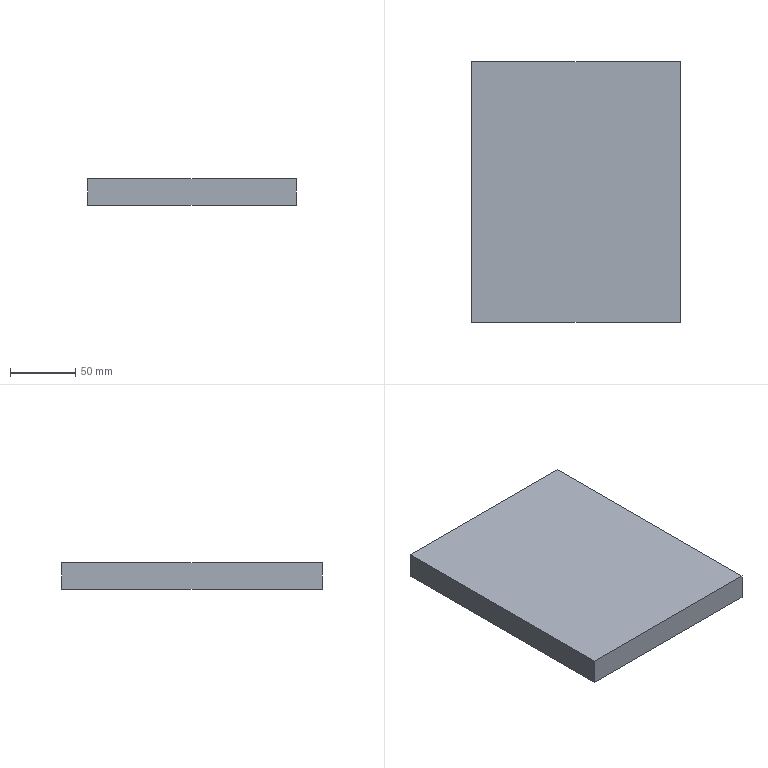Part | STEP file | Tube necking machine_id546_x_t | 1 solid | 6 faces | box 160 x 200 x 20 mm | volume 640000 mm3 | plane 6
STEP:
#1=CARTESIAN_POINT('',(0.,0.,0.));
#2=DIRECTION('',(0.,0.,1.));
#3=DIRECTION('',(1.,0.,0.));
#4=AXIS2_PLACEMENT_3D('',#1,#2,#3);
#5=CARTESIAN_POINT('',(387.5,150.,0.));
#6=VERTEX_POINT('',#5);
#7=CARTESIAN_POINT('',(387.5,-50.,0.));
#8=VERTEX_POINT('',#7);
#9=CARTESIAN_POINT('',(387.5,150.,0.));
#10=DIRECTION('',(0.,-1.,0.));
#11=VECTOR('',#10,1.);
#12=LINE('',#9,#11);
#13=CARTESIAN_POINT('',(387.5,150.,20.));
#14=DIRECTION('',(1.,0.,0.));
#15=DIRECTION('',(0.,0.,-1.));
#16=AXIS2_PLACEMENT_3D('',#13,#14,#15);
#17=PLANE('',#16);
#18=CARTESIAN_POINT('',(20.,0.));
#19=DIRECTION('',(0.,-1.));
#20=VECTOR('',#19,1.);
#21=LINE('',#18,#20);
#22=(GEOMETRIC_REPRESENTATION_CONTEXT(2)PARAMETRIC_REPRESENTATION_CONTEXT()REPRESENTATION_CONTEXT('',''));
#23=DEFINITIONAL_REPRESENTATION('',(#21),#22);
#24=PCURVE('',#17,#23);
#25=CARTESIAN_POINT('',(0.,0.,0.));
#26=DIRECTION('',(0.,0.,1.));
#27=DIRECTION('',(1.,0.,0.));
#28=AXIS2_PLACEMENT_3D('',#25,#26,#27);
#29=PLANE('',#28);
#30=CARTESIAN_POINT('',(387.5,150.));
#31=DIRECTION('',(0.,-1.));
#32=VECTOR('',#31,1.);
#33=LINE('',#30,#32);
#34=(GEOMETRIC_REPRESENTATION_CONTEXT(2)PARAMETRIC_REPRESENTATION_CONTEXT()REPRESENTATION_CONTEXT('',''));
#35=DEFINITIONAL_REPRESENTATION('',(#33),#34);
#36=PCURVE('',#29,#35);
#37=SURFACE_CURVE('',#12,(#24,#36),.PCURVE_S1.);
#38=EDGE_CURVE('',#6,#8,#37,.T.);
#39=ORIENTED_EDGE('',*,*,#38,.T.);
#40=CARTESIAN_POINT('',(387.5,-50.,20.));
#41=VERTEX_POINT('',#40);
#42=CARTESIAN_POINT('',(387.5,-50.,20.));
#43=DIRECTION('',(0.,0.,-1.));
#44=VECTOR('',#43,1.);
#45=LINE('',#42,#44);
#46=CARTESIAN_POINT('',(0.,-200.));
#47=DIRECTION('',(1.,0.));
#48=VECTOR('',#47,1.);
#49=LINE('',#46,#48);
#50=(GEOMETRIC_REPRESENTATION_CONTEXT(2)PARAMETRIC_REPRESENTATION_CONTEXT()REPRESENTATION_CONTEXT('',''));
#51=DEFINITIONAL_REPRESENTATION('',(#49),#50);
#52=PCURVE('',#17,#51);
#53=CARTESIAN_POINT('',(387.5,-50.,20.));
#54=DIRECTION('',(0.,1.,0.));
#55=DIRECTION('',(-1.,0.,0.));
#56=AXIS2_PLACEMENT_3D('',#53,#54,#55);
#57=PLANE('',#56);
#58=CARTESIAN_POINT('',(0.,0.));
#59=DIRECTION('',(0.,-1.));
#60=VECTOR('',#59,1.);
#61=LINE('',#58,#60);
#62=(GEOMETRIC_REPRESENTATION_CONTEXT(2)PARAMETRIC_REPRESENTATION_CONTEXT()REPRESENTATION_CONTEXT('',''));
#63=DEFINITIONAL_REPRESENTATION('',(#61),#62);
#64=PCURVE('',#57,#63);
#65=SURFACE_CURVE('',#45,(#52,#64),.PCURVE_S1.);
#66=EDGE_CURVE('',#41,#8,#65,.T.);
#67=ORIENTED_EDGE('',*,*,#66,.F.);
#68=CARTESIAN_POINT('',(387.5,150.,20.));
#69=VERTEX_POINT('',#68);
#70=CARTESIAN_POINT('',(387.5,150.,20.));
#71=DIRECTION('',(0.,-1.,0.));
#72=VECTOR('',#71,1.);
#73=LINE('',#70,#72);
#74=CARTESIAN_POINT('',(0.,0.));
#75=DIRECTION('',(0.,-1.));
#76=VECTOR('',#75,1.);
#77=LINE('',#74,#76);
#78=(GEOMETRIC_REPRESENTATION_CONTEXT(2)PARAMETRIC_REPRESENTATION_CONTEXT()REPRESENTATION_CONTEXT('',''));
#79=DEFINITIONAL_REPRESENTATION('',(#77),#78);
#80=PCURVE('',#17,#79);
#81=CARTESIAN_POINT('',(0.,0.,20.));
#82=DIRECTION('',(0.,0.,1.));
#83=DIRECTION('',(1.,0.,0.));
#84=AXIS2_PLACEMENT_3D('',#81,#82,#83);
#85=PLANE('',#84);
#86=CARTESIAN_POINT('',(387.5,150.));
#87=DIRECTION('',(0.,-1.));
#88=VECTOR('',#87,1.);
#89=LINE('',#86,#88);
#90=(GEOMETRIC_REPRESENTATION_CONTEXT(2)PARAMETRIC_REPRESENTATION_CONTEXT()REPRESENTATION_CONTEXT('',''));
#91=DEFINITIONAL_REPRESENTATION('',(#89),#90);
#92=PCURVE('',#85,#91);
#93=SURFACE_CURVE('',#73,(#80,#92),.PCURVE_S1.);
#94=EDGE_CURVE('',#69,#41,#93,.T.);
#95=ORIENTED_EDGE('',*,*,#94,.F.);
#96=CARTESIAN_POINT('',(387.5,150.,20.));
#97=DIRECTION('',(0.,0.,-1.));
#98=VECTOR('',#97,1.);
#99=LINE('',#96,#98);
#100=CARTESIAN_POINT('',(0.,0.));
#101=DIRECTION('',(1.,0.));
#102=VECTOR('',#101,1.);
#103=LINE('',#100,#102);
#104=(GEOMETRIC_REPRESENTATION_CONTEXT(2)PARAMETRIC_REPRESENTATION_CONTEXT()REPRESENTATION_CONTEXT('',''));
#105=DEFINITIONAL_REPRESENTATION('',(#103),#104);
#106=PCURVE('',#17,#105);
#107=CARTESIAN_POINT('',(547.5,150.,20.));
#108=DIRECTION('',(0.,-1.,0.));
#109=DIRECTION('',(0.,0.,-1.));
#110=AXIS2_PLACEMENT_3D('',#107,#108,#109);
#111=PLANE('',#110);
#112=CARTESIAN_POINT('',(0.,-160.));
#113=DIRECTION('',(1.,0.));
#114=VECTOR('',#113,1.);
#115=LINE('',#112,#114);
#116=(GEOMETRIC_REPRESENTATION_CONTEXT(2)PARAMETRIC_REPRESENTATION_CONTEXT()REPRESENTATION_CONTEXT('',''));
#117=DEFINITIONAL_REPRESENTATION('',(#115),#116);
#118=PCURVE('',#111,#117);
#119=SURFACE_CURVE('',#99,(#106,#118),.PCURVE_S1.);
#120=EDGE_CURVE('',#69,#6,#119,.T.);
#121=ORIENTED_EDGE('',*,*,#120,.T.);
#122=EDGE_LOOP('',(#39,#67,#95,#121));
#123=FACE_BOUND('',#122,.T.);
#124=ADVANCED_FACE('',(#123),#17,.F.);
#125=CARTESIAN_POINT('',(547.5,-50.,0.));
#126=VERTEX_POINT('',#125);
#127=CARTESIAN_POINT('',(387.5,-50.,0.));
#128=DIRECTION('',(1.,0.,0.));
#129=VECTOR('',#128,1.);
#130=LINE('',#127,#129);
#131=CARTESIAN_POINT('',(0.,-20.));
#132=DIRECTION('',(-1.,0.));
#133=VECTOR('',#132,1.);
#134=LINE('',#131,#133);
#135=(GEOMETRIC_REPRESENTATION_CONTEXT(2)PARAMETRIC_REPRESENTATION_CONTEXT()REPRESENTATION_CONTEXT('',''));
#136=DEFINITIONAL_REPRESENTATION('',(#134),#135);
#137=PCURVE('',#57,#136);
#138=CARTESIAN_POINT('',(387.5,-50.));
#139=DIRECTION('',(1.,0.));
#140=VECTOR('',#139,1.);
#141=LINE('',#138,#140);
#142=(GEOMETRIC_REPRESENTATION_CONTEXT(2)PARAMETRIC_REPRESENTATION_CONTEXT()REPRESENTATION_CONTEXT('',''));
#143=DEFINITIONAL_REPRESENTATION('',(#141),#142);
#144=PCURVE('',#29,#143);
#145=SURFACE_CURVE('',#130,(#137,#144),.PCURVE_S1.);
#146=EDGE_CURVE('',#8,#126,#145,.T.);
#147=ORIENTED_EDGE('',*,*,#146,.T.);
#148=CARTESIAN_POINT('',(547.5,-50.,20.));
#149=VERTEX_POINT('',#148);
#150=CARTESIAN_POINT('',(547.5,-50.,20.));
#151=DIRECTION('',(0.,0.,-1.));
#152=VECTOR('',#151,1.);
#153=LINE('',#150,#152);
#154=CARTESIAN_POINT('',(-160.,0.));
#155=DIRECTION('',(0.,-1.));
#156=VECTOR('',#155,1.);
#157=LINE('',#154,#156);
#158=(GEOMETRIC_REPRESENTATION_CONTEXT(2)PARAMETRIC_REPRESENTATION_CONTEXT()REPRESENTATION_CONTEXT('',''));
#159=DEFINITIONAL_REPRESENTATION('',(#157),#158);
#160=PCURVE('',#57,#159);
#161=CARTESIAN_POINT('',(547.5,-50.,20.));
#162=DIRECTION('',(-1.,0.,0.));
#163=DIRECTION('',(0.,-1.,0.));
#164=AXIS2_PLACEMENT_3D('',#161,#162,#163);
#165=PLANE('',#164);
#166=CARTESIAN_POINT('',(0.,0.));
#167=DIRECTION('',(0.,-1.));
#168=VECTOR('',#167,1.);
#169=LINE('',#166,#168);
#170=(GEOMETRIC_REPRESENTATION_CONTEXT(2)PARAMETRIC_REPRESENTATION_CONTEXT()REPRESENTATION_CONTEXT('',''));
#171=DEFINITIONAL_REPRESENTATION('',(#169),#170);
#172=PCURVE('',#165,#171);
#173=SURFACE_CURVE('',#153,(#160,#172),.PCURVE_S1.);
#174=EDGE_CURVE('',#149,#126,#173,.T.);
#175=ORIENTED_EDGE('',*,*,#174,.F.);
#176=CARTESIAN_POINT('',(387.5,-50.,20.));
#177=DIRECTION('',(1.,0.,0.));
#178=VECTOR('',#177,1.);
#179=LINE('',#176,#178);
#180=CARTESIAN_POINT('',(0.,0.));
#181=DIRECTION('',(-1.,0.));
#182=VECTOR('',#181,1.);
#183=LINE('',#180,#182);
#184=(GEOMETRIC_REPRESENTATION_CONTEXT(2)PARAMETRIC_REPRESENTATION_CONTEXT()REPRESENTATION_CONTEXT('',''));
#185=DEFINITIONAL_REPRESENTATION('',(#183),#184);
#186=PCURVE('',#57,#185);
#187=CARTESIAN_POINT('',(387.5,-50.));
#188=DIRECTION('',(1.,0.));
#189=VECTOR('',#188,1.);
#190=LINE('',#187,#189);
#191=(GEOMETRIC_REPRESENTATION_CONTEXT(2)PARAMETRIC_REPRESENTATION_CONTEXT()REPRESENTATION_CONTEXT('',''));
#192=DEFINITIONAL_REPRESENTATION('',(#190),#191);
#193=PCURVE('',#85,#192);
#194=SURFACE_CURVE('',#179,(#186,#193),.PCURVE_S1.);
#195=EDGE_CURVE('',#41,#149,#194,.T.);
#196=ORIENTED_EDGE('',*,*,#195,.F.);
#197=ORIENTED_EDGE('',*,*,#66,.T.);
#198=EDGE_LOOP('',(#147,#175,#196,#197));
#199=FACE_BOUND('',#198,.T.);
#200=ADVANCED_FACE('',(#199),#57,.F.);
#201=CARTESIAN_POINT('',(547.5,150.,0.));
#202=VERTEX_POINT('',#201);
#203=CARTESIAN_POINT('',(547.5,-50.,0.));
#204=DIRECTION('',(0.,1.,0.));
#205=VECTOR('',#204,1.);
#206=LINE('',#203,#205);
#207=CARTESIAN_POINT('',(0.,-20.));
#208=DIRECTION('',(-1.,0.));
#209=VECTOR('',#208,1.);
#210=LINE('',#207,#209);
#211=(GEOMETRIC_REPRESENTATION_CONTEXT(2)PARAMETRIC_REPRESENTATION_CONTEXT()REPRESENTATION_CONTEXT('',''));
#212=DEFINITIONAL_REPRESENTATION('',(#210),#211);
#213=PCURVE('',#165,#212);
#214=CARTESIAN_POINT('',(547.5,-50.));
#215=DIRECTION('',(0.,1.));
#216=VECTOR('',#215,1.);
#217=LINE('',#214,#216);
#218=(GEOMETRIC_REPRESENTATION_CONTEXT(2)PARAMETRIC_REPRESENTATION_CONTEXT()REPRESENTATION_CONTEXT('',''));
#219=DEFINITIONAL_REPRESENTATION('',(#217),#218);
#220=PCURVE('',#29,#219);
#221=SURFACE_CURVE('',#206,(#213,#220),.PCURVE_S1.);
#222=EDGE_CURVE('',#126,#202,#221,.T.);
#223=ORIENTED_EDGE('',*,*,#222,.T.);
#224=CARTESIAN_POINT('',(547.5,150.,20.));
#225=VERTEX_POINT('',#224);
#226=CARTESIAN_POINT('',(547.5,150.,20.));
#227=DIRECTION('',(0.,0.,-1.));
#228=VECTOR('',#227,1.);
#229=LINE('',#226,#228);
#230=CARTESIAN_POINT('',(-200.,0.));
#231=DIRECTION('',(0.,-1.));
#232=VECTOR('',#231,1.);
#233=LINE('',#230,#232);
#234=(GEOMETRIC_REPRESENTATION_CONTEXT(2)PARAMETRIC_REPRESENTATION_CONTEXT()REPRESENTATION_CONTEXT('',''));
#235=DEFINITIONAL_REPRESENTATION('',(#233),#234);
#236=PCURVE('',#165,#235);
#237=CARTESIAN_POINT('',(0.,0.));
#238=DIRECTION('',(1.,0.));
#239=VECTOR('',#238,1.);
#240=LINE('',#237,#239);
#241=(GEOMETRIC_REPRESENTATION_CONTEXT(2)PARAMETRIC_REPRESENTATION_CONTEXT()REPRESENTATION_CONTEXT('',''));
#242=DEFINITIONAL_REPRESENTATION('',(#240),#241);
#243=PCURVE('',#111,#242);
#244=SURFACE_CURVE('',#229,(#236,#243),.PCURVE_S1.);
#245=EDGE_CURVE('',#225,#202,#244,.T.);
#246=ORIENTED_EDGE('',*,*,#245,.F.);
#247=CARTESIAN_POINT('',(547.5,-50.,20.));
#248=DIRECTION('',(0.,1.,0.));
#249=VECTOR('',#248,1.);
#250=LINE('',#247,#249);
#251=CARTESIAN_POINT('',(0.,0.));
#252=DIRECTION('',(-1.,0.));
#253=VECTOR('',#252,1.);
#254=LINE('',#251,#253);
#255=(GEOMETRIC_REPRESENTATION_CONTEXT(2)PARAMETRIC_REPRESENTATION_CONTEXT()REPRESENTATION_CONTEXT('',''));
#256=DEFINITIONAL_REPRESENTATION('',(#254),#255);
#257=PCURVE('',#165,#256);
#258=CARTESIAN_POINT('',(547.5,-50.));
#259=DIRECTION('',(0.,1.));
#260=VECTOR('',#259,1.);
#261=LINE('',#258,#260);
#262=(GEOMETRIC_REPRESENTATION_CONTEXT(2)PARAMETRIC_REPRESENTATION_CONTEXT()REPRESENTATION_CONTEXT('',''));
#263=DEFINITIONAL_REPRESENTATION('',(#261),#262);
#264=PCURVE('',#85,#263);
#265=SURFACE_CURVE('',#250,(#257,#264),.PCURVE_S1.);
#266=EDGE_CURVE('',#149,#225,#265,.T.);
#267=ORIENTED_EDGE('',*,*,#266,.F.);
#268=ORIENTED_EDGE('',*,*,#174,.T.);
#269=EDGE_LOOP('',(#223,#246,#267,#268));
#270=FACE_BOUND('',#269,.T.);
#271=ADVANCED_FACE('',(#270),#165,.F.);
#272=CARTESIAN_POINT('',(547.5,150.,0.));
#273=DIRECTION('',(-1.,0.,0.));
#274=VECTOR('',#273,1.);
#275=LINE('',#272,#274);
#276=CARTESIAN_POINT('',(20.,0.));
#277=DIRECTION('',(0.,-1.));
#278=VECTOR('',#277,1.);
#279=LINE('',#276,#278);
#280=(GEOMETRIC_REPRESENTATION_CONTEXT(2)PARAMETRIC_REPRESENTATION_CONTEXT()REPRESENTATION_CONTEXT('',''));
#281=DEFINITIONAL_REPRESENTATION('',(#279),#280);
#282=PCURVE('',#111,#281);
#283=CARTESIAN_POINT('',(547.5,150.));
#284=DIRECTION('',(-1.,0.));
#285=VECTOR('',#284,1.);
#286=LINE('',#283,#285);
#287=(GEOMETRIC_REPRESENTATION_CONTEXT(2)PARAMETRIC_REPRESENTATION_CONTEXT()REPRESENTATION_CONTEXT('',''));
#288=DEFINITIONAL_REPRESENTATION('',(#286),#287);
#289=PCURVE('',#29,#288);
#290=SURFACE_CURVE('',#275,(#282,#289),.PCURVE_S1.);
#291=EDGE_CURVE('',#202,#6,#290,.T.);
#292=ORIENTED_EDGE('',*,*,#291,.T.);
#293=ORIENTED_EDGE('',*,*,#120,.F.);
#294=CARTESIAN_POINT('',(547.5,150.,20.));
#295=DIRECTION('',(-1.,0.,0.));
#296=VECTOR('',#295,1.);
#297=LINE('',#294,#296);
#298=CARTESIAN_POINT('',(0.,0.));
#299=DIRECTION('',(0.,-1.));
#300=VECTOR('',#299,1.);
#301=LINE('',#298,#300);
#302=(GEOMETRIC_REPRESENTATION_CONTEXT(2)PARAMETRIC_REPRESENTATION_CONTEXT()REPRESENTATION_CONTEXT('',''));
#303=DEFINITIONAL_REPRESENTATION('',(#301),#302);
#304=PCURVE('',#111,#303);
#305=CARTESIAN_POINT('',(547.5,150.));
#306=DIRECTION('',(-1.,0.));
#307=VECTOR('',#306,1.);
#308=LINE('',#305,#307);
#309=(GEOMETRIC_REPRESENTATION_CONTEXT(2)PARAMETRIC_REPRESENTATION_CONTEXT()REPRESENTATION_CONTEXT('',''));
#310=DEFINITIONAL_REPRESENTATION('',(#308),#309);
#311=PCURVE('',#85,#310);
#312=SURFACE_CURVE('',#297,(#304,#311),.PCURVE_S1.);
#313=EDGE_CURVE('',#225,#69,#312,.T.);
#314=ORIENTED_EDGE('',*,*,#313,.F.);
#315=ORIENTED_EDGE('',*,*,#245,.T.);
#316=EDGE_LOOP('',(#292,#293,#314,#315));
#317=FACE_BOUND('',#316,.T.);
#318=ADVANCED_FACE('',(#317),#111,.F.);
#319=ORIENTED_EDGE('',*,*,#94,.T.);
#320=ORIENTED_EDGE('',*,*,#195,.T.);
#321=ORIENTED_EDGE('',*,*,#266,.T.);
#322=ORIENTED_EDGE('',*,*,#313,.T.);
#323=EDGE_LOOP('',(#319,#320,#321,#322));
#324=FACE_BOUND('',#323,.T.);
#325=ADVANCED_FACE('',(#324),#85,.T.);
#326=ORIENTED_EDGE('',*,*,#38,.F.);
#327=ORIENTED_EDGE('',*,*,#291,.F.);
#328=ORIENTED_EDGE('',*,*,#222,.F.);
#329=ORIENTED_EDGE('',*,*,#146,.F.);
#330=EDGE_LOOP('',(#326,#327,#328,#329));
#331=FACE_BOUND('',#330,.T.);
#332=ADVANCED_FACE('',(#331),#29,.F.);
#333=CLOSED_SHELL('',(#124,#200,#271,#318,#325,#332));
#334=MANIFOLD_SOLID_BREP('',#333);
#335=(LENGTH_UNIT()NAMED_UNIT(*)SI_UNIT(.MILLI.,.METRE.));
#336=UNCERTAINTY_MEASURE_WITH_UNIT(LENGTH_MEASURE(0.0000001),#335,'','');
#337=(NAMED_UNIT(*)PLANE_ANGLE_UNIT()SI_UNIT($,.RADIAN.));
#338=(NAMED_UNIT(*)SI_UNIT($,.STERADIAN.)SOLID_ANGLE_UNIT());
#339=(GEOMETRIC_REPRESENTATION_CONTEXT(3)GLOBAL_UNCERTAINTY_ASSIGNED_CONTEXT((#336))GLOBAL_UNIT_ASSIGNED_CONTEXT((#335,#337,#338))REPRESENTATION_CONTEXT('',''));
#340=ADVANCED_BREP_SHAPE_REPRESENTATION('',(#4,#334),#339);